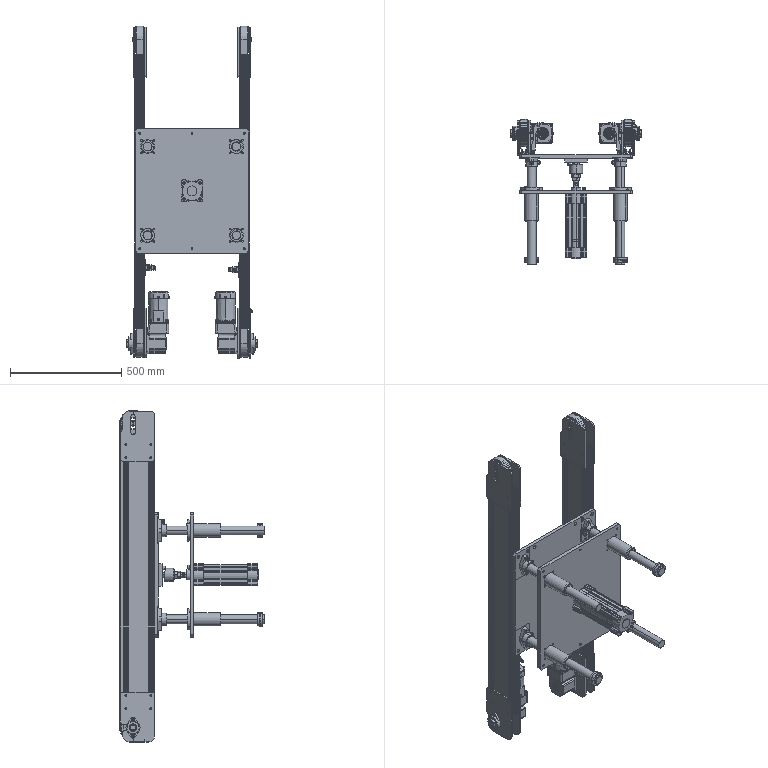Part | SolidWorks | 77 solids | 7179 faces | volume 25679072 mm3 | plane 3498 | cylinder 2730 | cone 379 | torus 340 | spline 184 | sphere 48 | commonest cylinder face diameters 1.6 x680 2 x224 112.75 x144 4 x110 8.5 x100 10 x98